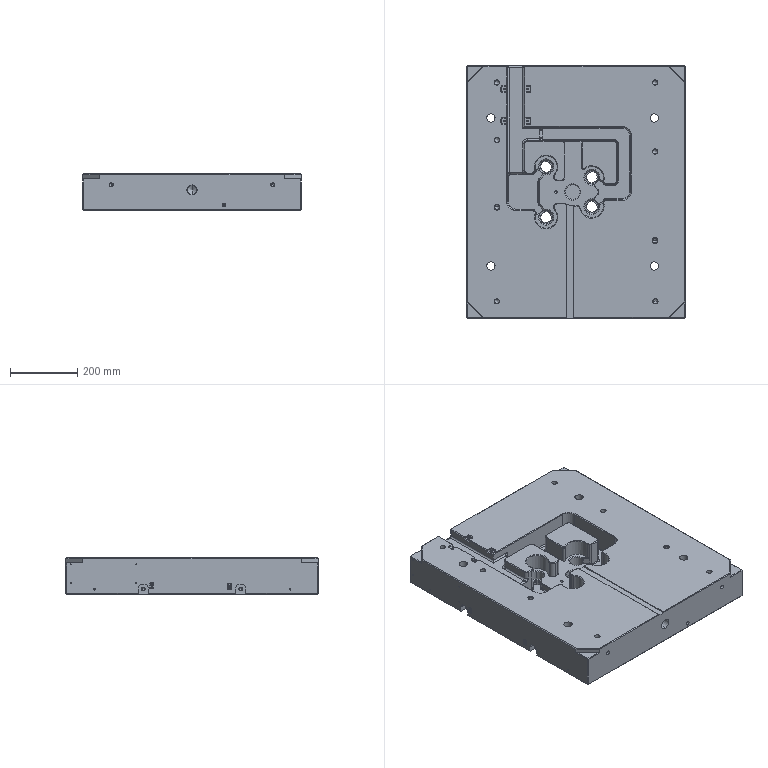Part | Creo | 1 solid | 967 faces | box 650 x 750 x 107.56 mm | volume 46977375 mm3 | plane 316 | cylinder 270 | cone 180 | other 154 | torus 41 | spline 6 | commonest cylinder face diameters 6 x33 16 x32 14 x28 20 x20 8 x18 5 x16